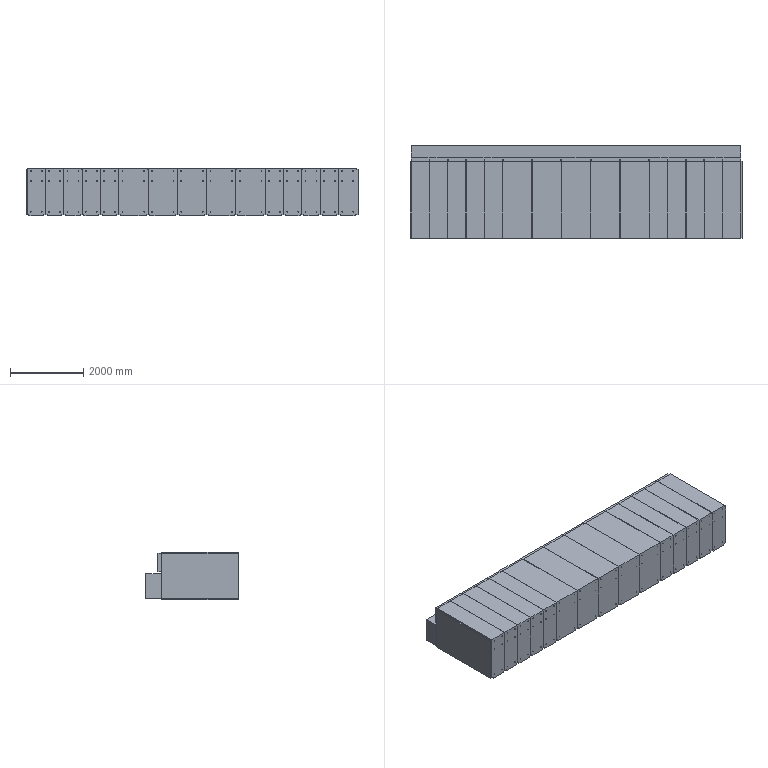Part | STEP file | 400-SW-102 | 29 solids | 751 faces | box 9074 x 2533 x 1310 mm | volume 27905066330 mm3 | plane 503 | cylinder 180 | spline 68 | commonest cylinder face diameters 20 x180